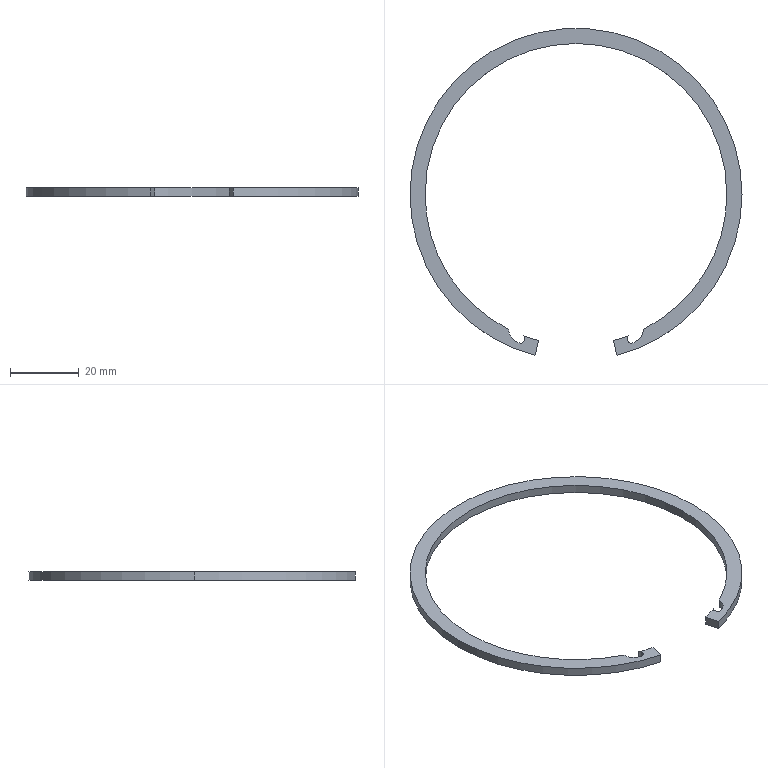Part | STEP file | Snap ring | 1 solid | 17 faces | box 96.5 x 95.005 x 2.5 mm | volume 2880 mm3 | cylinder 11 | plane 4 | spline 2 | commonest cylinder face diameters 87.7 x5 2.5 x3 96.5 x3
STEP:
#1=CARTESIAN_POINT('',(0.,0.,0.));
#2=DIRECTION('',(0.,0.,1.));
#3=DIRECTION('',(1.,0.,0.));
#4=AXIS2_PLACEMENT_3D('',#1,#2,#3);
#5=CARTESIAN_POINT('',(48.25,0.,2.5));
#6=VERTEX_POINT('',#5);
#7=CARTESIAN_POINT('',(-48.25,0.,2.5));
#8=VERTEX_POINT('',#7);
#9=CARTESIAN_POINT('',(0.,0.,2.5));
#10=DIRECTION('',(0.,0.,1.));
#11=DIRECTION('',(-1.,0.,0.));
#12=AXIS2_PLACEMENT_3D('',#9,#10,#11);
#13=CIRCLE('',#12,48.25);
#14=CARTESIAN_POINT('',(0.,0.,2.5));
#15=DIRECTION('',(0.,0.,-1.));
#16=DIRECTION('',(-1.,0.,0.));
#17=AXIS2_PLACEMENT_3D('',#14,#15,#16);
#18=CYLINDRICAL_SURFACE('',#17,48.25);
#19=CARTESIAN_POINT('',(6.283,0.));
#20=DIRECTION('',(-1.,0.));
#21=VECTOR('',#20,1.);
#22=LINE('',#19,#21);
#23=(GEOMETRIC_REPRESENTATION_CONTEXT(2)PARAMETRIC_REPRESENTATION_CONTEXT()REPRESENTATION_CONTEXT('',''));
#24=DEFINITIONAL_REPRESENTATION('',(#22),#23);
#25=PCURVE('',#18,#24);
#26=CARTESIAN_POINT('',(0.,0.,2.5));
#27=DIRECTION('',(0.,0.,1.));
#28=DIRECTION('',(1.,0.,0.));
#29=AXIS2_PLACEMENT_3D('',#26,#27,#28);
#30=PLANE('',#29);
#31=CARTESIAN_POINT('',(0.,0.));
#32=DIRECTION('',(-1.,0.));
#33=AXIS2_PLACEMENT_2D('',#31,#32);
#34=CIRCLE('',#33,48.25);
#35=(GEOMETRIC_REPRESENTATION_CONTEXT(2)PARAMETRIC_REPRESENTATION_CONTEXT()REPRESENTATION_CONTEXT('',''));
#36=DEFINITIONAL_REPRESENTATION('',(#34),#35);
#37=PCURVE('',#30,#36);
#38=SURFACE_CURVE('',#13,(#25,#37),.PCURVE_S1.);
#39=EDGE_CURVE('',#6,#8,#38,.T.);
#40=ORIENTED_EDGE('',*,*,#39,.F.);
#41=CARTESIAN_POINT('',(48.25,0.,0.));
#42=VERTEX_POINT('',#41);
#43=CARTESIAN_POINT('',(48.25,0.,2.5));
#44=DIRECTION('',(0.,0.,-1.));
#45=VECTOR('',#44,1.);
#46=LINE('',#43,#45);
#47=CARTESIAN_POINT('',(3.142,0.));
#48=DIRECTION('',(0.,1.));
#49=VECTOR('',#48,1.);
#50=LINE('',#47,#49);
#51=(GEOMETRIC_REPRESENTATION_CONTEXT(2)PARAMETRIC_REPRESENTATION_CONTEXT()REPRESENTATION_CONTEXT('',''));
#52=DEFINITIONAL_REPRESENTATION('',(#50),#51);
#53=PCURVE('',#18,#52);
#54=CARTESIAN_POINT('',(0.,0.,2.5));
#55=DIRECTION('',(0.,0.,-1.));
#56=DIRECTION('',(-1.,0.,0.));
#57=AXIS2_PLACEMENT_3D('',#54,#55,#56);
#58=CYLINDRICAL_SURFACE('',#57,48.25);
#59=CARTESIAN_POINT('',(3.142,0.));
#60=DIRECTION('',(0.,1.));
#61=VECTOR('',#60,1.);
#62=LINE('',#59,#61);
#63=(GEOMETRIC_REPRESENTATION_CONTEXT(2)PARAMETRIC_REPRESENTATION_CONTEXT()REPRESENTATION_CONTEXT('',''));
#64=DEFINITIONAL_REPRESENTATION('',(#62),#63);
#65=PCURVE('',#58,#64);
#66=SURFACE_CURVE('',#46,(#53,#65),.PCURVE_S1.);
#67=EDGE_CURVE('',#6,#42,#66,.T.);
#68=ORIENTED_EDGE('',*,*,#67,.T.);
#69=CARTESIAN_POINT('',(-48.25,0.,0.));
#70=VERTEX_POINT('',#69);
#71=CARTESIAN_POINT('',(0.,0.,0.));
#72=DIRECTION('',(0.,0.,1.));
#73=DIRECTION('',(-1.,0.,0.));
#74=AXIS2_PLACEMENT_3D('',#71,#72,#73);
#75=CIRCLE('',#74,48.25);
#76=CARTESIAN_POINT('',(6.283,2.5));
#77=DIRECTION('',(-1.,0.));
#78=VECTOR('',#77,1.);
#79=LINE('',#76,#78);
#80=(GEOMETRIC_REPRESENTATION_CONTEXT(2)PARAMETRIC_REPRESENTATION_CONTEXT()REPRESENTATION_CONTEXT('',''));
#81=DEFINITIONAL_REPRESENTATION('',(#79),#80);
#82=PCURVE('',#18,#81);
#83=CARTESIAN_POINT('',(0.,0.,0.));
#84=DIRECTION('',(0.,0.,1.));
#85=DIRECTION('',(1.,0.,0.));
#86=AXIS2_PLACEMENT_3D('',#83,#84,#85);
#87=PLANE('',#86);
#88=CARTESIAN_POINT('',(0.,0.));
#89=DIRECTION('',(-1.,0.));
#90=AXIS2_PLACEMENT_2D('',#88,#89);
#91=CIRCLE('',#90,48.25);
#92=(GEOMETRIC_REPRESENTATION_CONTEXT(2)PARAMETRIC_REPRESENTATION_CONTEXT()REPRESENTATION_CONTEXT('',''));
#93=DEFINITIONAL_REPRESENTATION('',(#91),#92);
#94=PCURVE('',#87,#93);
#95=SURFACE_CURVE('',#75,(#82,#94),.PCURVE_S1.);
#96=EDGE_CURVE('',#42,#70,#95,.T.);
#97=ORIENTED_EDGE('',*,*,#96,.T.);
#98=CARTESIAN_POINT('',(-48.25,0.,2.5));
#99=DIRECTION('',(0.,0.,-1.));
#100=VECTOR('',#99,1.);
#101=LINE('',#98,#100);
#102=CARTESIAN_POINT('',(0.,0.));
#103=DIRECTION('',(0.,1.));
#104=VECTOR('',#103,1.);
#105=LINE('',#102,#104);
#106=(GEOMETRIC_REPRESENTATION_CONTEXT(2)PARAMETRIC_REPRESENTATION_CONTEXT()REPRESENTATION_CONTEXT('',''));
#107=DEFINITIONAL_REPRESENTATION('',(#105),#106);
#108=PCURVE('',#18,#107);
#109=CARTESIAN_POINT('',(0.,0.,2.5));
#110=DIRECTION('',(0.,0.,-1.));
#111=DIRECTION('',(-1.,0.,0.));
#112=AXIS2_PLACEMENT_3D('',#109,#110,#111);
#113=CYLINDRICAL_SURFACE('',#112,48.25);
#114=CARTESIAN_POINT('',(6.283,0.));
#115=DIRECTION('',(0.,1.));
#116=VECTOR('',#115,1.);
#117=LINE('',#114,#116);
#118=(GEOMETRIC_REPRESENTATION_CONTEXT(2)PARAMETRIC_REPRESENTATION_CONTEXT()REPRESENTATION_CONTEXT('',''));
#119=DEFINITIONAL_REPRESENTATION('',(#117),#118);
#120=PCURVE('',#113,#119);
#121=SURFACE_CURVE('',#101,(#108,#120),.PCURVE_S1.);
#122=EDGE_CURVE('',#8,#70,#121,.T.);
#123=ORIENTED_EDGE('',*,*,#122,.F.);
#124=EDGE_LOOP('',(#40,#68,#97,#123));
#125=FACE_BOUND('',#124,.T.);
#126=ADVANCED_FACE('',(#125),#18,.T.);
#127=CARTESIAN_POINT('',(-11.918,-46.755,2.5));
#128=VERTEX_POINT('',#127);
#129=CARTESIAN_POINT('',(0.,0.,2.5));
#130=DIRECTION('',(0.,0.,1.));
#131=DIRECTION('',(-1.,0.,0.));
#132=AXIS2_PLACEMENT_3D('',#129,#130,#131);
#133=CIRCLE('',#132,48.25);
#134=CARTESIAN_POINT('',(6.283,0.));
#135=DIRECTION('',(-1.,0.));
#136=VECTOR('',#135,1.);
#137=LINE('',#134,#136);
#138=(GEOMETRIC_REPRESENTATION_CONTEXT(2)PARAMETRIC_REPRESENTATION_CONTEXT()REPRESENTATION_CONTEXT('',''));
#139=DEFINITIONAL_REPRESENTATION('',(#137),#138);
#140=PCURVE('',#113,#139);
#141=CARTESIAN_POINT('',(0.,0.));
#142=DIRECTION('',(-1.,0.));
#143=AXIS2_PLACEMENT_2D('',#141,#142);
#144=CIRCLE('',#143,48.25);
#145=(GEOMETRIC_REPRESENTATION_CONTEXT(2)PARAMETRIC_REPRESENTATION_CONTEXT()REPRESENTATION_CONTEXT('',''));
#146=DEFINITIONAL_REPRESENTATION('',(#144),#145);
#147=PCURVE('',#30,#146);
#148=SURFACE_CURVE('',#133,(#140,#147),.PCURVE_S1.);
#149=EDGE_CURVE('',#8,#128,#148,.T.);
#150=ORIENTED_EDGE('',*,*,#149,.F.);
#151=ORIENTED_EDGE('',*,*,#122,.T.);
#152=CARTESIAN_POINT('',(-11.918,-46.755,0.));
#153=VERTEX_POINT('',#152);
#154=CARTESIAN_POINT('',(0.,0.,0.));
#155=DIRECTION('',(0.,0.,1.));
#156=DIRECTION('',(-1.,0.,0.));
#157=AXIS2_PLACEMENT_3D('',#154,#155,#156);
#158=CIRCLE('',#157,48.25);
#159=CARTESIAN_POINT('',(6.283,2.5));
#160=DIRECTION('',(-1.,0.));
#161=VECTOR('',#160,1.);
#162=LINE('',#159,#161);
#163=(GEOMETRIC_REPRESENTATION_CONTEXT(2)PARAMETRIC_REPRESENTATION_CONTEXT()REPRESENTATION_CONTEXT('',''));
#164=DEFINITIONAL_REPRESENTATION('',(#162),#163);
#165=PCURVE('',#113,#164);
#166=CARTESIAN_POINT('',(0.,0.));
#167=DIRECTION('',(-1.,0.));
#168=AXIS2_PLACEMENT_2D('',#166,#167);
#169=CIRCLE('',#168,48.25);
#170=(GEOMETRIC_REPRESENTATION_CONTEXT(2)PARAMETRIC_REPRESENTATION_CONTEXT()REPRESENTATION_CONTEXT('',''));
#171=DEFINITIONAL_REPRESENTATION('',(#169),#170);
#172=PCURVE('',#87,#171);
#173=SURFACE_CURVE('',#158,(#165,#172),.PCURVE_S1.);
#174=EDGE_CURVE('',#70,#153,#173,.T.);
#175=ORIENTED_EDGE('',*,*,#174,.T.);
#176=CARTESIAN_POINT('',(-11.918,-46.755,2.5));
#177=DIRECTION('',(0.,0.,1.));
#178=VECTOR('',#177,1.);
#179=LINE('',#176,#178);
#180=CARTESIAN_POINT('',(4.962,0.));
#181=DIRECTION('',(0.,-1.));
#182=VECTOR('',#181,1.);
#183=LINE('',#180,#182);
#184=(GEOMETRIC_REPRESENTATION_CONTEXT(2)PARAMETRIC_REPRESENTATION_CONTEXT()REPRESENTATION_CONTEXT('',''));
#185=DEFINITIONAL_REPRESENTATION('',(#183),#184);
#186=PCURVE('',#113,#185);
#187=CARTESIAN_POINT('',(-10.831,-42.491,2.5));
#188=DIRECTION('',(-0.969,0.247,0.));
#189=DIRECTION('',(-0.247,-0.969,0.));
#190=AXIS2_PLACEMENT_3D('',#187,#188,#189);
#191=PLANE('',#190);
#192=CARTESIAN_POINT('',(4.4,0.));
#193=DIRECTION('',(0.,1.));
#194=VECTOR('',#193,1.);
#195=LINE('',#192,#194);
#196=(GEOMETRIC_REPRESENTATION_CONTEXT(2)PARAMETRIC_REPRESENTATION_CONTEXT()REPRESENTATION_CONTEXT('',''));
#197=DEFINITIONAL_REPRESENTATION('',(#195),#196);
#198=PCURVE('',#191,#197);
#199=SURFACE_CURVE('',#179,(#186,#198),.PCURVE_S1.);
#200=EDGE_CURVE('',#153,#128,#199,.T.);
#201=ORIENTED_EDGE('',*,*,#200,.T.);
#202=EDGE_LOOP('',(#150,#151,#175,#201));
#203=FACE_BOUND('',#202,.T.);
#204=ADVANCED_FACE('',(#203),#113,.T.);
#205=CARTESIAN_POINT('',(19.612,-39.22,0.));
#206=VERTEX_POINT('',#205);
#207=CARTESIAN_POINT('',(19.612,-39.22,2.5));
#208=VERTEX_POINT('',#207);
#209=CARTESIAN_POINT('',(19.612,-39.22,1.25));
#210=DIRECTION('',(0.,0.,1.));
#211=VECTOR('',#210,1.);
#212=LINE('',#209,#211);
#213=CARTESIAN_POINT('',(0.,0.,2.5));
#214=DIRECTION('',(0.,0.,-1.));
#215=DIRECTION('',(-1.,0.,0.));
#216=AXIS2_PLACEMENT_3D('',#213,#214,#215);
#217=CYLINDRICAL_SURFACE('',#216,43.85);
#218=CARTESIAN_POINT('',(4.249,1.25));
#219=DIRECTION('',(0.,-1.));
#220=VECTOR('',#219,1.);
#221=LINE('',#218,#220);
#222=(GEOMETRIC_REPRESENTATION_CONTEXT(2)PARAMETRIC_REPRESENTATION_CONTEXT()REPRESENTATION_CONTEXT('',''));
#223=DEFINITIONAL_REPRESENTATION('',(#221),#222);
#224=PCURVE('',#217,#223);
#225=CARTESIAN_POINT('',(16.56,-43.184,0.));
#226=CARTESIAN_POINT('',(16.56,-43.184,2.5));
#227=CARTESIAN_POINT('',(19.402,-42.149,0.));
#228=CARTESIAN_POINT('',(19.402,-42.149,2.5));
#229=CARTESIAN_POINT('',(19.612,-39.22,0.));
#230=CARTESIAN_POINT('',(19.612,-39.22,2.5));
#231=B_SPLINE_SURFACE_WITH_KNOTS('',2,1,((#225,#226),(#227,#228),(#229,#230)),.UNSPECIFIED.,.F.,.F.,.F.,(3,3),(2,2),(0.,1.),(0.,1.),.PIECEWISE_BEZIER_KNOTS.);
#232=CARTESIAN_POINT('',(1.,0.));
#233=CARTESIAN_POINT('',(1.,1.));
#234=B_SPLINE_CURVE_WITH_KNOTS('',1,(#232,#233),.UNSPECIFIED.,.F.,.F.,(2,2),(-1.25,1.25),.PIECEWISE_BEZIER_KNOTS.);
#235=(GEOMETRIC_REPRESENTATION_CONTEXT(2)PARAMETRIC_REPRESENTATION_CONTEXT()REPRESENTATION_CONTEXT('',''));
#236=DEFINITIONAL_REPRESENTATION('',(#234),#235);
#237=PCURVE('',#231,#236);
#238=SURFACE_CURVE('',#212,(#224,#237),.PCURVE_S1.);
#239=EDGE_CURVE('',#206,#208,#238,.T.);
#240=ORIENTED_EDGE('',*,*,#239,.F.);
#241=CARTESIAN_POINT('',(43.85,0.,0.));
#242=VERTEX_POINT('',#241);
#243=CARTESIAN_POINT('',(0.,0.,0.));
#244=DIRECTION('',(0.,0.,1.));
#245=DIRECTION('',(-1.,0.,0.));
#246=AXIS2_PLACEMENT_3D('',#243,#244,#245);
#247=CIRCLE('',#246,43.85);
#248=CARTESIAN_POINT('',(6.283,2.5));
#249=DIRECTION('',(-1.,0.));
#250=VECTOR('',#249,1.);
#251=LINE('',#248,#250);
#252=(GEOMETRIC_REPRESENTATION_CONTEXT(2)PARAMETRIC_REPRESENTATION_CONTEXT()REPRESENTATION_CONTEXT('',''));
#253=DEFINITIONAL_REPRESENTATION('',(#251),#252);
#254=PCURVE('',#217,#253);
#255=CARTESIAN_POINT('',(0.,0.));
#256=DIRECTION('',(-1.,0.));
#257=AXIS2_PLACEMENT_2D('',#255,#256);
#258=CIRCLE('',#257,43.85);
#259=(GEOMETRIC_REPRESENTATION_CONTEXT(2)PARAMETRIC_REPRESENTATION_CONTEXT()REPRESENTATION_CONTEXT('',''));
#260=DEFINITIONAL_REPRESENTATION('',(#258),#259);
#261=PCURVE('',#87,#260);
#262=SURFACE_CURVE('',#247,(#254,#261),.PCURVE_S1.);
#263=EDGE_CURVE('',#206,#242,#262,.T.);
#264=ORIENTED_EDGE('',*,*,#263,.T.);
#265=CARTESIAN_POINT('',(43.85,0.,2.5));
#266=VERTEX_POINT('',#265);
#267=CARTESIAN_POINT('',(43.85,0.,2.5));
#268=DIRECTION('',(0.,0.,-1.));
#269=VECTOR('',#268,1.);
#270=LINE('',#267,#269);
#271=CARTESIAN_POINT('',(3.142,0.));
#272=DIRECTION('',(0.,1.));
#273=VECTOR('',#272,1.);
#274=LINE('',#271,#273);
#275=(GEOMETRIC_REPRESENTATION_CONTEXT(2)PARAMETRIC_REPRESENTATION_CONTEXT()REPRESENTATION_CONTEXT('',''));
#276=DEFINITIONAL_REPRESENTATION('',(#274),#275);
#277=PCURVE('',#217,#276);
#278=CARTESIAN_POINT('',(0.,0.,2.5));
#279=DIRECTION('',(0.,0.,-1.));
#280=DIRECTION('',(-1.,0.,0.));
#281=AXIS2_PLACEMENT_3D('',#278,#279,#280);
#282=CYLINDRICAL_SURFACE('',#281,43.85);
#283=CARTESIAN_POINT('',(3.142,0.));
#284=DIRECTION('',(0.,1.));
#285=VECTOR('',#284,1.);
#286=LINE('',#283,#285);
#287=(GEOMETRIC_REPRESENTATION_CONTEXT(2)PARAMETRIC_REPRESENTATION_CONTEXT()REPRESENTATION_CONTEXT('',''));
#288=DEFINITIONAL_REPRESENTATION('',(#286),#287);
#289=PCURVE('',#282,#288);
#290=SURFACE_CURVE('',#270,(#277,#289),.PCURVE_S1.);
#291=EDGE_CURVE('',#266,#242,#290,.T.);
#292=ORIENTED_EDGE('',*,*,#291,.F.);
#293=CARTESIAN_POINT('',(0.,0.,2.5));
#294=DIRECTION('',(0.,0.,-1.));
#295=DIRECTION('',(-1.,0.,0.));
#296=AXIS2_PLACEMENT_3D('',#293,#294,#295);
#297=CIRCLE('',#296,43.85);
#298=CARTESIAN_POINT('',(0.,0.));
#299=DIRECTION('',(1.,0.));
#300=VECTOR('',#299,1.);
#301=LINE('',#298,#300);
#302=(GEOMETRIC_REPRESENTATION_CONTEXT(2)PARAMETRIC_REPRESENTATION_CONTEXT()REPRESENTATION_CONTEXT('',''));
#303=DEFINITIONAL_REPRESENTATION('',(#301),#302);
#304=PCURVE('',#217,#303);
#305=CARTESIAN_POINT('',(-43.85,0.));
#306=CARTESIAN_POINT('',(-43.85,75.95));
#307=CARTESIAN_POINT('',(21.925,37.975));
#308=CARTESIAN_POINT('',(87.7,0.));
#309=CARTESIAN_POINT('',(21.925,-37.975));
#310=CARTESIAN_POINT('',(-43.85,-75.95));
#311=CARTESIAN_POINT('',(-43.85,0.));
#312=(BOUNDED_CURVE()B_SPLINE_CURVE(2,(#305,#306,#307,#308,#309,#310,#311),.UNSPECIFIED.,.T.,.F.)B_SPLINE_CURVE_WITH_KNOTS((1,2,2,2,2,1),(-2.094,0.,2.094,4.189,6.283,8.378),.UNSPECIFIED.)CURVE()GEOMETRIC_REPRESENTATION_ITEM()RATIONAL_B_SPLINE_CURVE((1.,0.5,1.,0.5,1.,0.5,1.))REPRESENTATION_ITEM(''));
#313=(GEOMETRIC_REPRESENTATION_CONTEXT(2)PARAMETRIC_REPRESENTATION_CONTEXT()REPRESENTATION_CONTEXT('',''));
#314=DEFINITIONAL_REPRESENTATION('',(#312),#313);
#315=PCURVE('',#30,#314);
#316=SURFACE_CURVE('',#297,(#304,#315),.PCURVE_S1.);
#317=EDGE_CURVE('',#266,#208,#316,.T.);
#318=ORIENTED_EDGE('',*,*,#317,.T.);
#319=EDGE_LOOP('',(#240,#264,#292,#318));
#320=FACE_BOUND('',#319,.F.);
#321=ADVANCED_FACE('',(#320),#217,.F.);
#322=CARTESIAN_POINT('',(-43.85,0.,0.));
#323=VERTEX_POINT('',#322);
#324=CARTESIAN_POINT('',(0.,0.,0.));
#325=DIRECTION('',(0.,0.,1.));
#326=DIRECTION('',(-1.,0.,0.));
#327=AXIS2_PLACEMENT_3D('',#324,#325,#326);
#328=CIRCLE('',#327,43.85);
#329=CARTESIAN_POINT('',(6.283,2.5));
#330=DIRECTION('',(-1.,0.));
#331=VECTOR('',#330,1.);
#332=LINE('',#329,#331);
#333=(GEOMETRIC_REPRESENTATION_CONTEXT(2)PARAMETRIC_REPRESENTATION_CONTEXT()REPRESENTATION_CONTEXT('',''));
#334=DEFINITIONAL_REPRESENTATION('',(#332),#333);
#335=PCURVE('',#282,#334);
#336=CARTESIAN_POINT('',(0.,0.));
#337=DIRECTION('',(-1.,0.));
#338=AXIS2_PLACEMENT_2D('',#336,#337);
#339=CIRCLE('',#338,43.85);
#340=(GEOMETRIC_REPRESENTATION_CONTEXT(2)PARAMETRIC_REPRESENTATION_CONTEXT()REPRESENTATION_CONTEXT('',''));
#341=DEFINITIONAL_REPRESENTATION('',(#339),#340);
#342=PCURVE('',#87,#341);
#343=SURFACE_CURVE('',#328,(#335,#342),.PCURVE_S1.);
#344=EDGE_CURVE('',#242,#323,#343,.T.);
#345=ORIENTED_EDGE('',*,*,#344,.T.);
#346=CARTESIAN_POINT('',(-43.85,0.,2.5));
#347=VERTEX_POINT('',#346);
#348=CARTESIAN_POINT('',(-43.85,0.,2.5));
#349=DIRECTION('',(0.,0.,-1.));
#350=VECTOR('',#349,1.);
#351=LINE('',#348,#350);
#352=CARTESIAN_POINT('',(0.,0.));
#353=DIRECTION('',(0.,1.));
#354=VECTOR('',#353,1.);
#355=LINE('',#352,#354);
#356=(GEOMETRIC_REPRESENTATION_CONTEXT(2)PARAMETRIC_REPRESENTATION_CONTEXT()REPRESENTATION_CONTEXT('',''));
#357=DEFINITIONAL_REPRESENTATION('',(#355),#356);
#358=PCURVE('',#282,#357);
#359=CARTESIAN_POINT('',(0.,0.,2.5));
#360=DIRECTION('',(0.,0.,-1.));
#361=DIRECTION('',(-1.,0.,0.));
#362=AXIS2_PLACEMENT_3D('',#359,#360,#361);
#363=CYLINDRICAL_SURFACE('',#362,43.85);
#364=CARTESIAN_POINT('',(6.283,0.));
#365=DIRECTION('',(0.,1.));
#366=VECTOR('',#365,1.);
#367=LINE('',#364,#366);
#368=(GEOMETRIC_REPRESENTATION_CONTEXT(2)PARAMETRIC_REPRESENTATION_CONTEXT()REPRESENTATION_CONTEXT('',''));
#369=DEFINITIONAL_REPRESENTATION('',(#367),#368);
#370=PCURVE('',#363,#369);
#371=SURFACE_CURVE('',#351,(#358,#370),.PCURVE_S1.);
#372=EDGE_CURVE('',#347,#323,#371,.T.);
#373=ORIENTED_EDGE('',*,*,#372,.F.);
#374=CARTESIAN_POINT('',(0.,0.,2.5));
#375=DIRECTION('',(0.,0.,-1.));
#376=DIRECTION('',(-1.,0.,0.));
#377=AXIS2_PLACEMENT_3D('',#374,#375,#376);
#378=CIRCLE('',#377,43.85);
#379=CARTESIAN_POINT('',(0.,0.));
#380=DIRECTION('',(1.,0.));
#381=VECTOR('',#380,1.);
#382=LINE('',#379,#381);
#383=(GEOMETRIC_REPRESENTATION_CONTEXT(2)PARAMETRIC_REPRESENTATION_CONTEXT()REPRESENTATION_CONTEXT('',''));
#384=DEFINITIONAL_REPRESENTATION('',(#382),#383);
#385=PCURVE('',#282,#384);
#386=CARTESIAN_POINT('',(-43.85,0.));
#387=CARTESIAN_POINT('',(-43.85,75.95));
#388=CARTESIAN_POINT('',(21.925,37.975));
#389=CARTESIAN_POINT('',(87.7,0.));
#390=CARTESIAN_POINT('',(21.925,-37.975));
#391=CARTESIAN_POINT('',(-43.85,-75.95));
#392=CARTESIAN_POINT('',(-43.85,0.));
#393=(BOUNDED_CURVE()B_SPLINE_CURVE(2,(#386,#387,#388,#389,#390,#391,#392),.UNSPECIFIED.,.T.,.F.)B_SPLINE_CURVE_WITH_KNOTS((1,2,2,2,2,1),(-2.094,0.,2.094,4.189,6.283,8.378),.UNSPECIFIED.)CURVE()GEOMETRIC_REPRESENTATION_ITEM()RATIONAL_B_SPLINE_CURVE((1.,0.5,1.,0.5,1.,0.5,1.))REPRESENTATION_ITEM(''));
#394=(GEOMETRIC_REPRESENTATION_CONTEXT(2)PARAMETRIC_REPRESENTATION_CONTEXT()REPRESENTATION_CONTEXT('',''));
#395=DEFINITIONAL_REPRESENTATION('',(#393),#394);
#396=PCURVE('',#30,#395);
#397=SURFACE_CURVE('',#378,(#385,#396),.PCURVE_S1.);
#398=EDGE_CURVE('',#347,#266,#397,.T.);
#399=ORIENTED_EDGE('',*,*,#398,.T.);
#400=ORIENTED_EDGE('',*,*,#291,.T.);
#401=EDGE_LOOP('',(#345,#373,#399,#400));
#402=FACE_BOUND('',#401,.F.);
#403=ADVANCED_FACE('',(#402),#282,.F.);
#404=CARTESIAN_POINT('',(-15.262,-41.108,2.5));
#405=VERTEX_POINT('',#404);
#406=CARTESIAN_POINT('',(-15.262,-41.108,0.));
#407=VERTEX_POINT('',#406);
#408=CARTESIAN_POINT('',(-15.262,-41.108,2.5));
#409=DIRECTION('',(0.,0.,-1.));
#410=VECTOR('',#409,1.);
#411=LINE('',#408,#410);
#412=CARTESIAN_POINT('',(-16.126,-42.011,0.));
#413=DIRECTION('',(0.,0.,1.));
#414=DIRECTION('',(1.,0.,0.));
#415=AXIS2_PLACEMENT_3D('',#412,#413,#414);
#416=CYLINDRICAL_SURFACE('',#415,1.25);
#417=CARTESIAN_POINT('',(0.807,2.5));
#418=DIRECTION('',(0.,-1.));
#419=VECTOR('',#418,1.);
#420=LINE('',#417,#419);
#421=(GEOMETRIC_REPRESENTATION_CONTEXT(2)PARAMETRIC_REPRESENTATION_CONTEXT()REPRESENTATION_CONTEXT('',''));
#422=DEFINITIONAL_REPRESENTATION('',(#420),#421);
#423=PCURVE('',#416,#422);
#424=CARTESIAN_POINT('',(0.,0.,2.5));
#425=DIRECTION('',(0.,0.,-1.));
#426=DIRECTION('',(-1.,0.,0.));
#427=AXIS2_PLACEMENT_3D('',#424,#425,#426);
#428=CYLINDRICAL_SURFACE('',#427,43.85);
#429=CARTESIAN_POINT('',(5.068,0.));
#430=DIRECTION('',(0.,1.));
#431=VECTOR('',#430,1.);
#432=LINE('',#429,#431);
#433=(GEOMETRIC_REPRESENTATION_CONTEXT(2)PARAMETRIC_REPRESENTATION_CONTEXT()REPRESENTATION_CONTEXT('',''));
#434=DEFINITIONAL_REPRESENTATION('',(#432),#433);
#435=PCURVE('',#428,#434);
#436=SURFACE_CURVE('',#411,(#423,#435),.PCURVE_S1.);
#437=EDGE_CURVE('',#405,#407,#436,.T.);
#438=ORIENTED_EDGE('',*,*,#437,.F.);
#439=CARTESIAN_POINT('',(-14.876,-42.011,2.5));
#440=VERTEX_POINT('',#439);
#441=CARTESIAN_POINT('',(-16.126,-42.011,2.5));
#442=DIRECTION('',(0.,0.,-1.));
#443=DIRECTION('',(1.,0.,0.));
#444=AXIS2_PLACEMENT_3D('',#441,#442,#443);
#445=CIRCLE('',#444,1.25);
#446=CARTESIAN_POINT('',(6.283,2.5));
#447=DIRECTION('',(-1.,0.));
#448=VECTOR('',#447,1.);
#449=LINE('',#446,#448);
#450=(GEOMETRIC_REPRESENTATION_CONTEXT(2)PARAMETRIC_REPRESENTATION_CONTEXT()REPRESENTATION_CONTEXT('',''));
#451=DEFINITIONAL_REPRESENTATION('',(#449),#450);
#452=PCURVE('',#416,#451);
#453=CARTESIAN_POINT('',(-14.876,-42.011));
#454=CARTESIAN_POINT('',(-14.876,-44.176));
#455=CARTESIAN_POINT('',(-16.751,-43.094));
#456=CARTESIAN_POINT('',(-18.626,-42.011));
#457=CARTESIAN_POINT('',(-16.751,-40.929));
#458=CARTESIAN_POINT('',(-14.876,-39.846));
#459=CARTESIAN_POINT('',(-14.876,-42.011));
#460=(BOUNDED_CURVE()B_SPLINE_CURVE(2,(#453,#454,#455,#456,#457,#458,#459),.UNSPECIFIED.,.T.,.F.)B_SPLINE_CURVE_WITH_KNOTS((1,2,2,2,2,1),(-2.094,0.,2.094,4.189,6.283,8.378),.UNSPECIFIED.)CURVE()GEOMETRIC_REPRESENTATION_ITEM()RATIONAL_B_SPLINE_CURVE((1.,0.5,1.,0.5,1.,0.5,1.))REPRESENTATION_ITEM(''));
#461=(GEOMETRIC_REPRESENTATION_CONTEXT(2)PARAMETRIC_REPRESENTATION_CONTEXT()REPRESENTATION_CONTEXT('',''));
#462=DEFINITIONAL_REPRESENTATION('',(#460),#461);
#463=PCURVE('',#30,#462);
#464=SURFACE_CURVE('',#445,(#452,#463),.PCURVE_S1.);
#465=EDGE_CURVE('',#405,#440,#464,.T.);
#466=ORIENTED_EDGE('',*,*,#465,.T.);
#467=CARTESIAN_POINT('',(-14.876,-42.011,0.));
#468=VERTEX_POINT('',#467);
#469=CARTESIAN_POINT('',(-14.876,-42.011,0.));
#470=DIRECTION('',(0.,0.,1.));
#471=VECTOR('',#470,1.);
#472=LINE('',#469,#471);
#473=CARTESIAN_POINT('',(0.,0.));
#474=DIRECTION('',(0.,1.));
#475=VECTOR('',#474,1.);
#476=LINE('',#473,#475);
#477=(GEOMETRIC_REPRESENTATION_CONTEXT(2)PARAMETRIC_REPRESENTATION_CONTEXT()REPRESENTATION_CONTEXT('',''));
#478=DEFINITIONAL_REPRESENTATION('',(#476),#477);
#479=PCURVE('',#416,#478);
#480=CARTESIAN_POINT('',(-16.126,-42.011,0.));
#481=DIRECTION('',(0.,0.,1.));
#482=DIRECTION('',(1.,0.,0.));
#483=AXIS2_PLACEMENT_3D('',#480,#481,#482);
#484=CYLINDRICAL_SURFACE('',#483,1.25);
#485=CARTESIAN_POINT('',(6.283,0.));
#486=DIRECTION('',(0.,1.));
#487=VECTOR('',#486,1.);
#488=LINE('',#485,#487);
#489=(GEOMETRIC_REPRESENTATION_CONTEXT(2)PARAMETRIC_REPRESENTATION_CONTEXT()REPRESENTATION_CONTEXT('',''));
#490=DEFINITIONAL_REPRESENTATION('',(#488),#489);
#491=PCURVE('',#484,#490);
#492=SURFACE_CURVE('',#472,(#479,#491),.PCURVE_S1.);
#493=EDGE_CURVE('',#468,#440,#492,.T.);
#494=ORIENTED_EDGE('',*,*,#493,.F.);
#495=CARTESIAN_POINT('',(-16.126,-42.011,0.));
#496=DIRECTION('',(0.,0.,1.));
#497=DIRECTION('',(1.,0.,0.));
#498=AXIS2_PLACEMENT_3D('',#495,#496,#497);
#499=CIRCLE('',#498,1.25);
#500=CARTESIAN_POINT('',(0.,0.));
#501=DIRECTION('',(1.,0.));
#502=VECTOR('',#501,1.);
#503=LINE('',#500,#502);
#504=(GEOMETRIC_REPRESENTATION_CONTEXT(2)PARAMETRIC_REPRESENTATION_CONTEXT()REPRESENTATION_CONTEXT('',''));
#505=DEFINITIONAL_REPRESENTATION('',(#503),#504);
#506=PCURVE('',#416,#505);
#507=CARTESIAN_POINT('',(-16.126,-42.011));
#508=DIRECTION('',(1.,0.));
#509=AXIS2_PLACEMENT_2D('',#507,#508);
#510=CIRCLE('',#509,1.25);
#511=(GEOMETRIC_REPRESENTATION_CONTEXT(2)PARAMETRIC_REPRESENTATION_CONTEXT()REPRESENTATION_CONTEXT('',''));
#512=DEFINITIONAL_REPRESENTATION('',(#510),#511);
#513=PCURVE('',#87,#512);
#514=SURFACE_CURVE('',#499,(#506,#513),.PCURVE_S1.);
#515=EDGE_CURVE('',#468,#407,#514,.T.);
#516=ORIENTED_EDGE('',*,*,#515,.T.);
#517=EDGE_LOOP('',(#438,#466,#494,#516));
#518=FACE_BOUND('',#517,.F.);
#519=ADVANCED_FACE('',(#518),#416,.F.);
#520=CARTESIAN_POINT('',(-10.831,-42.491,2.5));
#521=VERTEX_POINT('',#520);
#522=CARTESIAN_POINT('',(-11.918,-46.755,2.5));
#523=DIRECTION('',(0.247,0.969,0.));
#524=VECTOR('',#523,1.);
#525=LINE('',#522,#524);
#526=CARTESIAN_POINT('',(-11.918,-46.755));
#527=DIRECTION('',(0.247,0.969));
#528=VECTOR('',#527,1.);
#529=LINE('',#526,#528);
#530=(GEOMETRIC_REPRESENTATION_CONTEXT(2)PARAMETRIC_REPRESENTATION_CONTEXT()REPRESENTATION_CONTEXT('',''));
#531=DEFINITIONAL_REPRESENTATION('',(#529),#530);
#532=PCURVE('',#30,#531);
#533=CARTESIAN_POINT('',(4.4,0.));
#534=DIRECTION('',(-1.,0.));
#535=VECTOR('',#534,1.);
#536=LINE('',#533,#535);
#537=(GEOMETRIC_REPRESENTATION_CONTEXT(2)PARAMETRIC_REPRESENTATION_CONTEXT()REPRESENTATION_CONTEXT('',''));
#538=DEFINITIONAL_REPRESENTATION('',(#536),#537);
#539=PCURVE('',#191,#538);
#540=SURFACE_CURVE('',#525,(#532,#539),.PCURVE_S1.);
#541=EDGE_CURVE('',#128,#521,#540,.T.);
#542=ORIENTED_EDGE('',*,*,#541,.T.);
#543=CARTESIAN_POINT('',(0.,0.,2.5));
#544=DIRECTION('',(0.,0.,-1.));
#545=DIRECTION('',(-1.,0.,0.));
#546=AXIS2_PLACEMENT_3D('',#543,#544,#545);
#547=CIRCLE('',#546,43.85);
#548=CARTESIAN_POINT('',(-43.85,0.));
#549=CARTESIAN_POINT('',(-43.85,75.95));
#550=CARTESIAN_POINT('',(21.925,37.975));
#551=CARTESIAN_POINT('',(87.7,0.));
#552=CARTESIAN_POINT('',(21.925,-37.975));
#553=CARTESIAN_POINT('',(-43.85,-75.95));
#554=CARTESIAN_POINT('',(-43.85,0.));
#555=(BOUNDED_CURVE()B_SPLINE_CURVE(2,(#548,#549,#550,#551,#552,#553,#554),.UNSPECIFIED.,.T.,.F.)B_SPLINE_CURVE_WITH_KNOTS((1,2,2,2,2,1),(-2.094,0.,2.094,4.189,6.283,8.378),.UNSPECIFIED.)CURVE()GEOMETRIC_REPRESENTATION_ITEM()RATIONAL_B_SPLINE_CURVE((1.,0.5,1.,0.5,1.,0.5,1.))REPRESENTATION_ITEM(''));
#556=(GEOMETRIC_REPRESENTATION_CONTEXT(2)PARAMETRIC_REPRESENTATION_CONTEXT()REPRESENTATION_CONTEXT('',''));
#557=DEFINITIONAL_REPRESENTATION('',(#555),#556);
#558=PCURVE('',#30,#557);
#559=CARTESIAN_POINT('',(0.,0.));
#560=DIRECTION('',(1.,0.));
#561=VECTOR('',#560,1.);
#562=LINE('',#559,#561);
#563=(GEOMETRIC_REPRESENTATION_CONTEXT(2)PARAMETRIC_REPRESENTATION_CONTEXT()REPRESENTATION_CONTEXT('',''));
#564=DEFINITIONAL_REPRESENTATION('',(#562),#563);
#565=PCURVE('',#428,#564);
#566=SURFACE_CURVE('',#547,(#558,#565),.PCURVE_S1.);
#567=EDGE_CURVE('',#521,#405,#566,.T.);
#568=ORIENTED_EDGE('',*,*,#567,.T.);
#569=ORIENTED_EDGE('',*,*,#465,.T.);
#570=CARTESIAN_POINT('',(-16.56,-43.184,2.5));
#571=VERTEX_POINT('',#570);
#572=CARTESIAN_POINT('',(-16.126,-42.011,2.5));
#573=DIRECTION('',(0.,0.,-1.));
#574=DIRECTION('',(1.,0.,0.));
#575=AXIS2_PLACEMENT_3D('',#572,#573,#574);
#576=CIRCLE('',#575,1.25);
#577=CARTESIAN_POINT('',(-14.876,-42.011));
#578=CARTESIAN_POINT('',(-14.876,-44.176));
#579=CARTESIAN_POINT('',(-16.751,-43.094));
#580=CARTESIAN_POINT('',(-18.626,-42.011));
#581=CARTESIAN_POINT('',(-16.751,-40.929));
#582=CARTESIAN_POINT('',(-14.876,-39.846));
#583=CARTESIAN_POINT('',(-14.876,-42.011));
#584=(BOUNDED_CURVE()B_SPLINE_CURVE(2,(#577,#578,#579,#580,#581,#582,#583),.UNSPECIFIED.,.T.,.F.)B_SPLINE_CURVE_WITH_KNOTS((1,2,2,2,2,1),(-2.094,0.,2.094,4.189,6.283,8.378),.UNSPECIFIED.)CURVE()GEOMETRIC_REPRESENTATION_ITEM()RATIONAL_B_SPLINE_CURVE((1.,0.5,1.,0.5,1.,0.5,1.))REPRESENTATION_ITEM(''));
#585=(GEOMETRIC_REPRESENTATION_CONTEXT(2)PARAMETRIC_REPRESENTATION_CONTEXT()REPRESENTATION_CONTEXT('',''));
#586=DEFINITIONAL_REPRESENTATION('',(#584),#585);
#587=PCURVE('',#30,#586);
#588=CARTESIAN_POINT('',(6.283,2.5));
#589=DIRECTION('',(-1.,0.));
#590=VECTOR('',#589,1.);
#591=LINE('',#588,#590);
#592=(GEOMETRIC_REPRESENTATION_CONTEXT(2)PARAMETRIC_REPRESENTATION_CONTEXT()REPRESENTATION_CONTEXT('',''));
#593=DEFINITIONAL_REPRESENTATION('',(#591),#592);
#594=PCURVE('',#484,#593);
#595=SURFACE_CURVE('',#576,(#587,#594),.PCURVE_S1.);
#596=EDGE_CURVE('',#440,#571,#595,.T.);
#597=ORIENTED_EDGE('',*,*,#596,.T.);
#598=CARTESIAN_POINT('',(-19.612,-39.22,2.5));
#599=VERTEX_POINT('',#598);
#600=CARTESIAN_POINT('',(-16.56,-43.184,2.5));
#601=CARTESIAN_POINT('',(-18.454,-42.494,2.5));
#602=CARTESIAN_POINT('',(-19.472,-41.173,2.5));
#603=CARTESIAN_POINT('',(-19.612,-39.22,2.5));
#604=B_SPLINE_CURVE_WITH_KNOTS('',3,(#600,#601,#602,#603),.UNSPECIFIED.,.F.,.F.,(4,4),(0.,1.),.PIECEWISE_BEZIER_KNOTS.);
#605=CARTESIAN_POINT('',(-16.56,-43.184));
#606=CARTESIAN_POINT('',(-18.454,-42.494));
#607=CARTESIAN_POINT('',(-19.472,-41.173));
#608=CARTESIAN_POINT('',(-19.612,-39.22));
#609=B_SPLINE_CURVE_WITH_KNOTS('',3,(#605,#606,#607,#608),.UNSPECIFIED.,.F.,.F.,(4,4),(0.,1.),.PIECEWISE_BEZIER_KNOTS.);
#610=(GEOMETRIC_REPRESENTATION_CONTEXT(2)PARAMETRIC_REPRESENTATION_CONTEXT()REPRESENTATION_CONTEXT('',''));
#611=DEFINITIONAL_REPRESENTATION('',(#609),#610);
#612=PCURVE('',#30,#611);
#613=CARTESIAN_POINT('',(-16.56,-43.184,0.));
#614=CARTESIAN_POINT('',(-16.56,-43.184,2.5));
#615=CARTESIAN_POINT('',(-19.402,-42.149,0.));
#616=CARTESIAN_POINT('',(-19.402,-42.149,2.5));
#617=CARTESIAN_POINT('',(-19.612,-39.22,0.));
#618=CARTESIAN_POINT('',(-19.612,-39.22,2.5));
#619=B_SPLINE_SURFACE_WITH_KNOTS('',2,1,((#613,#614),(#615,#616),(#617,#618)),.UNSPECIFIED.,.F.,.F.,.F.,(3,3),(2,2),(0.,1.),(0.,1.),.PIECEWISE_BEZIER_KNOTS.);
#620=CARTESIAN_POINT('',(0.,1.));
#621=DIRECTION('',(1.,0.));
#622=VECTOR('',#621,1.);
#623=LINE('',#620,#622);
#624=(GEOMETRIC_REPRESENTATION_CONTEXT(2)PARAMETRIC_REPRESENTATION_CONTEXT()REPRESENTATION_CONTEXT('',''));
#625=DEFINITIONAL_REPRESENTATION('',(#623),#624);
#626=PCURVE('',#619,#625);
#627=SURFACE_CURVE('',#604,(#612,#626),.PCURVE_S1.);
#628=EDGE_CURVE('',#571,#599,#627,.T.);
#629=ORIENTED_EDGE('',*,*,#628,.T.);
#630=CARTESIAN_POINT('',(0.,0.,2.5));
#631=DIRECTION('',(0.,0.,-1.));
#632=DIRECTION('',(-1.,0.,0.));
#633=AXIS2_PLACEMENT_3D('',#630,#631,#632);
#634=CIRCLE('',#633,43.85);
#635=CARTESIAN_POINT('',(-43.85,0.));
#636=CARTESIAN_POINT('',(-43.85,75.95));
#637=CARTESIAN_POINT('',(21.925,37.975));
#638=CARTESIAN_POINT('',(87.7,0.));
#639=CARTESIAN_POINT('',(21.925,-37.975));
#640=CARTESIAN_POINT('',(-43.85,-75.95));
#641=CARTESIAN_POINT('',(-43.85,0.));
#642=(BOUNDED_CURVE()B_SPLINE_CURVE(2,(#635,#636,#637,#638,#639,#640,#641),.UNSPECIFIED.,.T.,.F.)B_SPLINE_CURVE_WITH_KNOTS((1,2,2,2,2,1),(-2.094,0.,2.094,4.189,6.283,8.378),.UNSPECIFIED.)CURVE()GEOMETRIC_REPRESENTATION_ITEM()RATIONAL_B_SPLINE_CURVE((1.,0.5,1.,0.5,1.,0.5,1.))REPRESENTATION_ITEM(''));
#643=(GEOMETRIC_REPRESENTATION_CONTEXT(2)PARAMETRIC_REPRESENTATION_CONTEXT()REPRESENTATION_CONTEXT('',''));
#644=DEFINITIONAL_REPRESENTATION('',(#642),#643);
#645=PCURVE('',#30,#644);
#646=CARTESIAN_POINT('',(0.,0.));
#647=DIRECTION('',(1.,0.));
#648=VECTOR('',#647,1.);
#649=LINE('',#646,#648);
#650=(GEOMETRIC_REPRESENTATION_CONTEXT(2)PARAMETRIC_REPRESENTATION_CONTEXT()REPRESENTATION_CONTEXT('',''));
#651=DEFINITIONAL_REPRESENTATION('',(#649),#650);
#652=PCURVE('',#363,#651);
#653=SURFACE_CURVE('',#634,(#645,#652),.PCURVE_S1.);
#654=EDGE_CURVE('',#599,#347,#653,.T.);
#655=ORIENTED_EDGE('',*,*,#654,.T.);
#656=ORIENTED_EDGE('',*,*,#398,.T.);
#657=ORIENTED_EDGE('',*,*,#317,.T.);
#658=CARTESIAN_POINT('',(16.56,-43.184,2.5));
#659=VERTEX_POINT('',#658);
#660=CARTESIAN_POINT('',(19.612,-39.22,2.5));
#661=CARTESIAN_POINT('',(19.472,-41.173,2.5));
#662=CARTESIAN_POINT('',(18.454,-42.494,2.5));
#663=CARTESIAN_POINT('',(16.56,-43.184,2.5));
#664=B_SPLINE_CURVE_WITH_KNOTS('',3,(#660,#661,#662,#663),.UNSPECIFIED.,.F.,.F.,(4,4),(0.,1.),.PIECEWISE_BEZIER_KNOTS.);
#665=CARTESIAN_POINT('',(19.612,-39.22));
#666=CARTESIAN_POINT('',(19.472,-41.173));
#667=CARTESIAN_POINT('',(18.454,-42.494));
#668=CARTESIAN_POINT('',(16.56,-43.184));
#669=B_SPLINE_CURVE_WITH_KNOTS('',3,(#665,#666,#667,#668),.UNSPECIFIED.,.F.,.F.,(4,4),(0.,1.),.PIECEWISE_BEZIER_KNOTS.);
#670=(GEOMETRIC_REPRESENTATION_CONTEXT(2)PARAMETRIC_REPRESENTATION_CONTEXT()REPRESENTATION_CONTEXT('',''));
#671=DEFINITIONAL_REPRESENTATION('',(#669),#670);
#672=PCURVE('',#30,#671);
#673=CARTESIAN_POINT('',(1.,1.));
#674=DIRECTION('',(-1.,0.));
#675=VECTOR('',#674,1.);
#676=LINE('',#673,#675);
#677=(GEOMETRIC_REPRESENTATION_CONTEXT(2)PARAMETRIC_REPRESENTATION_CONTEXT()REPRESENTATION_CONTEXT('',''));
#678=DEFINITIONAL_REPRESENTATION('',(#676),#677);
#679=PCURVE('',#231,#678);
#680=SURFACE_CURVE('',#664,(#672,#679),.PCURVE_S1.);
#681=EDGE_CURVE('',#208,#659,#680,.T.);
#682=ORIENTED_EDGE('',*,*,#681,.T.);
#683=CARTESIAN_POINT('',(15.262,-41.108,2.5));
#684=VERTEX_POINT('',#683);
#685=CARTESIAN_POINT('',(16.126,-42.011,2.5));
#686=DIRECTION('',(0.,0.,-1.));
#687=DIRECTION('',(1.,0.,0.));
#688=AXIS2_PLACEMENT_3D('',#685,#686,#687);
#689=CIRCLE('',#688,1.25);
#690=CARTESIAN_POINT('',(17.376,-42.011));
#691=CARTESIAN_POINT('',(17.376,-44.176));
#692=CARTESIAN_POINT('',(15.501,-43.094));
#693=CARTESIAN_POINT('',(13.626,-42.011));
#694=CARTESIAN_POINT('',(15.501,-40.929));
#695=CARTESIAN_POINT('',(17.376,-39.846));
#696=CARTESIAN_POINT('',(17.376,-42.011));
#697=(BOUNDED_CURVE()B_SPLINE_CURVE(2,(#690,#691,#692,#693,#694,#695,#696),.UNSPECIFIED.,.T.,.F.)B_SPLINE_CURVE_WITH_KNOTS((1,2,2,2,2,1),(-2.094,0.,2.094,4.189,6.283,8.378),.UNSPECIFIED.)CURVE()GEOMETRIC_REPRESENTATION_ITEM()RATIONAL_B_SPLINE_CURVE((1.,0.5,1.,0.5,1.,0.5,1.))REPRESENTATION_ITEM(''));
#698=(GEOMETRIC_REPRESENTATION_CONTEXT(2)PARAMETRIC_REPRESENTATION_CONTEXT()REPRESENTATION_CONTEXT('',''));
#699=DEFINITIONAL_REPRESENTATION('',(#697),#698);
#700=PCURVE('',#30,#699);
#701=CARTESIAN_POINT('',(16.126,-42.011,0.));
#702=DIRECTION('',(0.,0.,1.));
#703=DIRECTION('',(1.,0.,0.));
#704=AXIS2_PLACEMENT_3D('',#701,#702,#703);
#705=CYLINDRICAL_SURFACE('',#704,1.25);
#706=CARTESIAN_POINT('',(6.283,2.5));
#707=DIRECTION('',(-1.,0.));
#708=VECTOR('',#707,1.);
#709=LINE('',#706,#708);
#710=(GEOMETRIC_REPRESENTATION_CONTEXT(2)PARAMETRIC_REPRESENTATION_CONTEXT()REPRESENTATION_CONTEXT('',''));
#711=DEFINITIONAL_REPRESENTATION('',(#709),#710);
#712=PCURVE('',#705,#711);
#713=SURFACE_CURVE('',#689,(#700,#712),.PCURVE_S1.);
#714=EDGE_CURVE('',#659,#684,#713,.T.);
#715=ORIENTED_EDGE('',*,*,#714,.T.);
#716=CARTESIAN_POINT('',(10.831,-42.491,2.5));
#717=VERTEX_POINT('',#716);
#718=CARTESIAN_POINT('',(0.,0.,2.5));
#719=DIRECTION('',(0.,0.,-1.));
#720=DIRECTION('',(-1.,0.,0.));
#721=AXIS2_PLACEMENT_3D('',#718,#719,#720);
#722=CIRCLE('',#721,43.85);
#723=CARTESIAN_POINT('',(-43.85,0.));
#724=CARTESIAN_POINT('',(-43.85,75.95));
#725=CARTESIAN_POINT('',(21.925,37.975));
#726=CARTESIAN_POINT('',(87.7,0.));
#727=CARTESIAN_POINT('',(21.925,-37.975));
#728=CARTESIAN_POINT('',(-43.85,-75.95));
#729=CARTESIAN_POINT('',(-43.85,0.));
#730=(BOUNDED_CURVE()B_SPLINE_CURVE(2,(#723,#724,#725,#726,#727,#728,#729),.UNSPECIFIED.,.T.,.F.)B_SPLINE_CURVE_WITH_KNOTS((1,2,2,2,2,1),(-2.094,0.,2.094,4.189,6.283,8.378),.UNSPECIFIED.)CURVE()GEOMETRIC_REPRESENTATION_ITEM()RATIONAL_B_SPLINE_CURVE((1.,0.5,1.,0.5,1.,0.5,1.))REPRESENTATION_ITEM(''));
#731=(GEOMETRIC_REPRESENTATION_CONTEXT(2)PARAMETRIC_REPRESENTATION_CONTEXT()REPRESENTATION_CONTEXT('',''));
#732=DEFINITIONAL_REPRESENTATION('',(#730),#731);
#733=PCURVE('',#30,#732);
#734=CARTESIAN_POINT('',(0.,0.,2.5));
#735=DIRECTION('',(0.,0.,-1.));
#736=DIRECTION('',(-1.,0.,0.));
#737=AXIS2_PLACEMENT_3D('',#734,#735,#736);
#738=CYLINDRICAL_SURFACE('',#737,43.85);
#739=CARTESIAN_POINT('',(0.,0.));
#740=DIRECTION('',(1.,0.));
#741=VECTOR('',#740,1.);
#742=LINE('',#739,#741);
#743=(GEOMETRIC_REPRESENTATION_CONTEXT(2)PARAMETRIC_REPRESENTATION_CONTEXT()REPRESENTATION_CONTEXT('',''));
#744=DEFINITIONAL_REPRESENTATION('',(#742),#743);
#745=PCURVE('',#738,#744);
#746=SURFACE_CURVE('',#722,(#733,#745),.PCURVE_S1.);
#747=EDGE_CURVE('',#684,#717,#746,.T.);
#748=ORIENTED_EDGE('',*,*,#747,.T.);
#749=CARTESIAN_POINT('',(11.918,-46.755,2.5));
#750=VERTEX_POINT('',#749);
#751=CARTESIAN_POINT('',(10.831,-42.491,2.5));
#752=DIRECTION('',(0.247,-0.969,0.));
#753=VECTOR('',#752,1.);
#754=LINE('',#751,#753);
#755=CARTESIAN_POINT('',(10.831,-42.491));
#756=DIRECTION('',(0.247,-0.969));
#757=VECTOR('',#756,1.);
#758=LINE('',#755,#757);
#759=(GEOMETRIC_REPRESENTATION_CONTEXT(2)PARAMETRIC_REPRESENTATION_CONTEXT()REPRESENTATION_CONTEXT('',''));
#760=DEFINITIONAL_REPRESENTATION('',(#758),#759);
#761=PCURVE('',#30,#760);
#762=CARTESIAN_POINT('',(10.831,-42.491,2.5));
#763=DIRECTION('',(0.969,0.247,0.));
#764=DIRECTION('',(-0.247,0.969,0.));
#765=AXIS2_PLACEMENT_3D('',#762,#763,#764);
#766=PLANE('',#765);
#767=CARTESIAN_POINT('',(0.,0.));
#768=DIRECTION('',(-1.,0.));
#769=VECTOR('',#768,1.);
#770=LINE('',#767,#769);
#771=(GEOMETRIC_REPRESENTATION_CONTEXT(2)PARAMETRIC_REPRESENTATION_CONTEXT()REPRESENTATION_CONTEXT('',''));
#772=DEFINITIONAL_REPRESENTATION('',(#770),#771);
#773=PCURVE('',#766,#772);
#774=SURFACE_CURVE('',#754,(#761,#773),.PCURVE_S1.);
#775=EDGE_CURVE('',#717,#750,#774,.T.);
#776=ORIENTED_EDGE('',*,*,#775,.T.);
#777=CARTESIAN_POINT('',(0.,0.,2.5));
#778=DIRECTION('',(0.,0.,1.));
#779=DIRECTION('',(-1.,0.,0.));
#780=AXIS2_PLACEMENT_3D('',#777,#778,#779);
#781=CIRCLE('',#780,48.25);
#782=CARTESIAN_POINT('',(0.,0.));
#783=DIRECTION('',(-1.,0.));
#784=AXIS2_PLACEMENT_2D('',#782,#783);
#785=CIRCLE('',#784,48.25);
#786=(GEOMETRIC_REPRESENTATION_CONTEXT(2)PARAMETRIC_REPRESENTATION_CONTEXT()REPRESENTATION_CONTEXT('',''));
#787=DEFINITIONAL_REPRESENTATION('',(#785),#786);
#788=PCURVE('',#30,#787);
#789=CARTESIAN_POINT('',(6.283,0.));
#790=DIRECTION('',(-1.,0.));
#791=VECTOR('',#790,1.);
#792=LINE('',#789,#791);
#793=(GEOMETRIC_REPRESENTATION_CONTEXT(2)PARAMETRIC_REPRESENTATION_CONTEXT()REPRESENTATION_CONTEXT('',''));
#794=DEFINITIONAL_REPRESENTATION('',(#792),#793);
#795=PCURVE('',#58,#794);
#796=SURFACE_CURVE('',#781,(#788,#795),.PCURVE_S1.);
#797=EDGE_CURVE('',#750,#6,#796,.T.);
#798=ORIENTED_EDGE('',*,*,#797,.T.);
#799=ORIENTED_EDGE('',*,*,#39,.T.);
#800=ORIENTED_EDGE('',*,*,#149,.T.);
#801=EDGE_LOOP('',(#542,#568,#569,#597,#629,#655,#656,#657,#682,#715,#748,#776,#798,#799,#800));
#802=FACE_BOUND('',#801,.T.);
#803=ADVANCED_FACE('',(#802),#30,.T.);
#804=ORIENTED_EDGE('',*,*,#437,.T.);
#805=CARTESIAN_POINT('',(-10.831,-42.491,0.));
#806=VERTEX_POINT('',#805);
#807=CARTESIAN_POINT('',(0.,0.,0.));
#808=DIRECTION('',(0.,0.,1.));
#809=DIRECTION('',(-1.,0.,0.));
#810=AXIS2_PLACEMENT_3D('',#807,#808,#809);
#811=CIRCLE('',#810,43.85);
#812=CARTESIAN_POINT('',(6.283,2.5));
#813=DIRECTION('',(-1.,0.));
#814=VECTOR('',#813,1.);
#815=LINE('',#812,#814);
#816=(GEOMETRIC_REPRESENTATION_CONTEXT(2)PARAMETRIC_REPRESENTATION_CONTEXT()REPRESENTATION_CONTEXT('',''));
#817=DEFINITIONAL_REPRESENTATION('',(#815),#816);
#818=PCURVE('',#428,#817);
#819=CARTESIAN_POINT('',(0.,0.));
#820=DIRECTION('',(-1.,0.));
#821=AXIS2_PLACEMENT_2D('',#819,#820);
#822=CIRCLE('',#821,43.85);
#823=(GEOMETRIC_REPRESENTATION_CONTEXT(2)PARAMETRIC_REPRESENTATION_CONTEXT()REPRESENTATION_CONTEXT('',''));
#824=DEFINITIONAL_REPRESENTATION('',(#822),#823);
#825=PCURVE('',#87,#824);
#826=SURFACE_CURVE('',#811,(#818,#825),.PCURVE_S1.);
#827=EDGE_CURVE('',#407,#806,#826,.T.);
#828=ORIENTED_EDGE('',*,*,#827,.T.);
#829=CARTESIAN_POINT('',(-10.831,-42.491,2.5));
#830=DIRECTION('',(0.,0.,1.));
#831=VECTOR('',#830,1.);
#832=LINE('',#829,#831);
#833=CARTESIAN_POINT('',(4.962,0.));
#834=DIRECTION('',(0.,-1.));
#835=VECTOR('',#834,1.);
#836=LINE('',#833,#835);
#837=(GEOMETRIC_REPRESENTATION_CONTEXT(2)PARAMETRIC_REPRESENTATION_CONTEXT()REPRESENTATION_CONTEXT('',''));
#838=DEFINITIONAL_REPRESENTATION('',(#836),#837);
#839=PCURVE('',#428,#838);
#840=CARTESIAN_POINT('',(0.,0.));
#841=DIRECTION('',(0.,1.));
#842=VECTOR('',#841,1.);
#843=LINE('',#840,#842);
#844=(GEOMETRIC_REPRESENTATION_CONTEXT(2)PARAMETRIC_REPRESENTATION_CONTEXT()REPRESENTATION_CONTEXT('',''));
#845=DEFINITIONAL_REPRESENTATION('',(#843),#844);
#846=PCURVE('',#191,#845);
#847=SURFACE_CURVE('',#832,(#839,#846),.PCURVE_S1.);
#848=EDGE_CURVE('',#806,#521,#847,.T.);
#849=ORIENTED_EDGE('',*,*,#848,.T.);
#850=ORIENTED_EDGE('',*,*,#567,.T.);
#851=EDGE_LOOP('',(#804,#828,#849,#850));
#852=FACE_BOUND('',#851,.F.);
#853=ADVANCED_FACE('',(#852),#428,.F.);
#854=ORIENTED_EDGE('',*,*,#848,.T.);
#855=ORIENTED_EDGE('',*,*,#541,.F.);
#856=ORIENTED_EDGE('',*,*,#200,.F.);
#857=CARTESIAN_POINT('',(-10.831,-42.491,0.));
#858=DIRECTION('',(-0.247,-0.969,0.));
#859=VECTOR('',#858,1.);
#860=LINE('',#857,#859);
#861=CARTESIAN_POINT('',(0.,-2.5));
#862=DIRECTION('',(1.,0.));
#863=VECTOR('',#862,1.);
#864=LINE('',#861,#863);
#865=(GEOMETRIC_REPRESENTATION_CONTEXT(2)PARAMETRIC_REPRESENTATION_CONTEXT()REPRESENTATION_CONTEXT('',''));
#866=DEFINITIONAL_REPRESENTATION('',(#864),#865);
#867=PCURVE('',#191,#866);
#868=CARTESIAN_POINT('',(-10.831,-42.491));
#869=DIRECTION('',(-0.247,-0.969));
#870=VECTOR('',#869,1.);
#871=LINE('',#868,#870);
#872=(GEOMETRIC_REPRESENTATION_CONTEXT(2)PARAMETRIC_REPRESENTATION_CONTEXT()REPRESENTATION_CONTEXT('',''));
#873=DEFINITIONAL_REPRESENTATION('',(#871),#872);
#874=PCURVE('',#87,#873);
#875=SURFACE_CURVE('',#860,(#867,#874),.PCURVE_S1.);
#876=EDGE_CURVE('',#806,#153,#875,.T.);
#877=ORIENTED_EDGE('',*,*,#876,.F.);
#878=EDGE_LOOP('',(#854,#855,#856,#877));
#879=FACE_BOUND('',#878,.T.);
#880=ADVANCED_FACE('',(#879),#191,.F.);
#881=ORIENTED_EDGE('',*,*,#67,.F.);
#882=ORIENTED_EDGE('',*,*,#797,.F.);
#883=CARTESIAN_POINT('',(11.918,-46.755,0.));
#884=VERTEX_POINT('',#883);
#885=CARTESIAN_POINT('',(11.918,-46.755,2.5));
#886=DIRECTION('',(0.,0.,-1.));
#887=VECTOR('',#886,1.);
#888=LINE('',#885,#887);
#889=CARTESIAN_POINT('',(4.463,0.));
#890=DIRECTION('',(0.,1.));
#891=VECTOR('',#890,1.);
#892=LINE('',#889,#891);
#893=(GEOMETRIC_REPRESENTATION_CONTEXT(2)PARAMETRIC_REPRESENTATION_CONTEXT()REPRESENTATION_CONTEXT('',''));
#894=DEFINITIONAL_REPRESENTATION('',(#892),#893);
#895=PCURVE('',#58,#894);
#896=CARTESIAN_POINT('',(-4.4,0.));
#897=DIRECTION('',(0.,-1.));
#898=VECTOR('',#897,1.);
#899=LINE('',#896,#898);
#900=(GEOMETRIC_REPRESENTATION_CONTEXT(2)PARAMETRIC_REPRESENTATION_CONTEXT()REPRESENTATION_CONTEXT('',''));
#901=DEFINITIONAL_REPRESENTATION('',(#899),#900);
#902=PCURVE('',#766,#901);
#903=SURFACE_CURVE('',#888,(#895,#902),.PCURVE_S1.);
#904=EDGE_CURVE('',#750,#884,#903,.T.);
#905=ORIENTED_EDGE('',*,*,#904,.T.);
#906=CARTESIAN_POINT('',(0.,0.,0.));
#907=DIRECTION('',(0.,0.,1.));
#908=DIRECTION('',(-1.,0.,0.));
#909=AXIS2_PLACEMENT_3D('',#906,#907,#908);
#910=CIRCLE('',#909,48.25);
#911=CARTESIAN_POINT('',(6.283,2.5));
#912=DIRECTION('',(-1.,0.));
#913=VECTOR('',#912,1.);
#914=LINE('',#911,#913);
#915=(GEOMETRIC_REPRESENTATION_CONTEXT(2)PARAMETRIC_REPRESENTATION_CONTEXT()REPRESENTATION_CONTEXT('',''));
#916=DEFINITIONAL_REPRESENTATION('',(#914),#915);
#917=PCURVE('',#58,#916);
#918=CARTESIAN_POINT('',(0.,0.));
#919=DIRECTION('',(-1.,0.));
#920=AXIS2_PLACEMENT_2D('',#918,#919);
#921=CIRCLE('',#920,48.25);
#922=(GEOMETRIC_REPRESENTATION_CONTEXT(2)PARAMETRIC_REPRESENTATION_CONTEXT()REPRESENTATION_CONTEXT('',''));
#923=DEFINITIONAL_REPRESENTATION('',(#921),#922);
#924=PCURVE('',#87,#923);
#925=SURFACE_CURVE('',#910,(#917,#924),.PCURVE_S1.);
#926=EDGE_CURVE('',#884,#42,#925,.T.);
#927=ORIENTED_EDGE('',*,*,#926,.T.);
#928=EDGE_LOOP('',(#881,#882,#905,#927));
#929=FACE_BOUND('',#928,.T.);
#930=ADVANCED_FACE('',(#929),#58,.T.);
#931=ORIENTED_EDGE('',*,*,#904,.F.);
#932=ORIENTED_EDGE('',*,*,#775,.F.);
#933=CARTESIAN_POINT('',(10.831,-42.491,0.));
#934=VERTEX_POINT('',#933);
#935=CARTESIAN_POINT('',(10.831,-42.491,2.5));
#936=DIRECTION('',(0.,0.,1.));
#937=VECTOR('',#936,1.);
#938=LINE('',#935,#937);
#939=CARTESIAN_POINT('',(0.,0.));
#940=DIRECTION('',(0.,1.));
#941=VECTOR('',#940,1.);
#942=LINE('',#939,#941);
#943=(GEOMETRIC_REPRESENTATION_CONTEXT(2)PARAMETRIC_REPRESENTATION_CONTEXT()REPRESENTATION_CONTEXT('',''));
#944=DEFINITIONAL_REPRESENTATION('',(#942),#943);
#945=PCURVE('',#766,#944);
#946=CARTESIAN_POINT('',(4.463,0.));
#947=DIRECTION('',(0.,-1.));
#948=VECTOR('',#947,1.);
#949=LINE('',#946,#948);
#950=(GEOMETRIC_REPRESENTATION_CONTEXT(2)PARAMETRIC_REPRESENTATION_CONTEXT()REPRESENTATION_CONTEXT('',''));
#951=DEFINITIONAL_REPRESENTATION('',(#949),#950);
#952=PCURVE('',#738,#951);
#953=SURFACE_CURVE('',#938,(#945,#952),.PCURVE_S1.);
#954=EDGE_CURVE('',#934,#717,#953,.T.);
#955=ORIENTED_EDGE('',*,*,#954,.F.);
#956=CARTESIAN_POINT('',(10.831,-42.491,0.));
#957=DIRECTION('',(-0.247,0.969,0.));
#958=VECTOR('',#957,1.);
#959=LINE('',#956,#958);
#960=CARTESIAN_POINT('',(0.,-2.5));
#961=DIRECTION('',(1.,0.));
#962=VECTOR('',#961,1.);
#963=LINE('',#960,#962);
#964=(GEOMETRIC_REPRESENTATION_CONTEXT(2)PARAMETRIC_REPRESENTATION_CONTEXT()REPRESENTATION_CONTEXT('',''));
#965=DEFINITIONAL_REPRESENTATION('',(#963),#964);
#966=PCURVE('',#766,#965);
#967=CARTESIAN_POINT('',(10.831,-42.491));
#968=DIRECTION('',(-0.247,0.969));
#969=VECTOR('',#968,1.);
#970=LINE('',#967,#969);
#971=(GEOMETRIC_REPRESENTATION_CONTEXT(2)PARAMETRIC_REPRESENTATION_CONTEXT()REPRESENTATION_CONTEXT('',''));
#972=DEFINITIONAL_REPRESENTATION('',(#970),#971);
#973=PCURVE('',#87,#972);
#974=SURFACE_CURVE('',#959,(#966,#973),.PCURVE_S1.);
#975=EDGE_CURVE('',#884,#934,#974,.T.);
#976=ORIENTED_EDGE('',*,*,#975,.F.);
#977=EDGE_LOOP('',(#931,#932,#955,#976));
#978=FACE_BOUND('',#977,.T.);
#979=ADVANCED_FACE('',(#978),#766,.F.);
#980=ORIENTED_EDGE('',*,*,#747,.T.);
#981=ORIENTED_EDGE('',*,*,#954,.F.);
#982=CARTESIAN_POINT('',(15.262,-41.108,0.));
#983=VERTEX_POINT('',#982);
#984=CARTESIAN_POINT('',(0.,0.,0.));
#985=DIRECTION('',(0.,0.,1.));
#986=DIRECTION('',(-1.,0.,0.));
#987=AXIS2_PLACEMENT_3D('',#984,#985,#986);
#988=CIRCLE('',#987,43.85);
#989=CARTESIAN_POINT('',(6.283,2.5));
#990=DIRECTION('',(-1.,0.));
#991=VECTOR('',#990,1.);
#992=LINE('',#989,#991);
#993=(GEOMETRIC_REPRESENTATION_CONTEXT(2)PARAMETRIC_REPRESENTATION_CONTEXT()REPRESENTATION_CONTEXT('',''));
#994=DEFINITIONAL_REPRESENTATION('',(#992),#993);
#995=PCURVE('',#738,#994);
#996=CARTESIAN_POINT('',(0.,0.));
#997=DIRECTION('',(-1.,0.));
#998=AXIS2_PLACEMENT_2D('',#996,#997);
#999=CIRCLE('',#998,43.85);
#1000=(GEOMETRIC_REPRESENTATION_CONTEXT(2)PARAMETRIC_REPRESENTATION_CONTEXT()REPRESENTATION_CONTEXT('',''));
#1001=DEFINITIONAL_REPRESENTATION('',(#999),#1000);
#1002=PCURVE('',#87,#1001);
#1003=SURFACE_CURVE('',#988,(#995,#1002),.PCURVE_S1.);
#1004=EDGE_CURVE('',#934,#983,#1003,.T.);
#1005=ORIENTED_EDGE('',*,*,#1004,.T.);
#1006=CARTESIAN_POINT('',(15.262,-41.108,2.5));
#1007=DIRECTION('',(0.,0.,1.));
#1008=VECTOR('',#1007,1.);
#1009=LINE('',#1006,#1008);
#1010=CARTESIAN_POINT('',(4.357,0.));
#1011=DIRECTION('',(0.,-1.));
#1012=VECTOR('',#1011,1.);
#1013=LINE('',#1010,#1012);
#1014=(GEOMETRIC_REPRESENTATION_CONTEXT(2)PARAMETRIC_REPRESENTATION_CONTEXT()REPRESENTATION_CONTEXT('',''));
#1015=DEFINITIONAL_REPRESENTATION('',(#1013),#1014);
#1016=PCURVE('',#738,#1015);
#1017=CARTESIAN_POINT('',(2.335,2.5));
#1018=DIRECTION('',(0.,1.));
#1019=VECTOR('',#1018,1.);
#1020=LINE('',#1017,#1019);
#1021=(GEOMETRIC_REPRESENTATION_CONTEXT(2)PARAMETRIC_REPRESENTATION_CONTEXT()REPRESENTATION_CONTEXT('',''));
#1022=DEFINITIONAL_REPRESENTATION('',(#1020),#1021);
#1023=PCURVE('',#705,#1022);
#1024=SURFACE_CURVE('',#1009,(#1016,#1023),.PCURVE_S1.);
#1025=EDGE_CURVE('',#983,#684,#1024,.T.);
#1026=ORIENTED_EDGE('',*,*,#1025,.T.);
#1027=EDGE_LOOP('',(#980,#981,#1005,#1026));
#1028=FACE_BOUND('',#1027,.F.);
#1029=ADVANCED_FACE('',(#1028),#738,.F.);
#1030=ORIENTED_EDGE('',*,*,#714,.T.);
#1031=ORIENTED_EDGE('',*,*,#1025,.F.);
#1032=CARTESIAN_POINT('',(16.56,-43.184,0.));
#1033=VERTEX_POINT('',#1032);
#1034=CARTESIAN_POINT('',(16.126,-42.011,0.));
#1035=DIRECTION('',(0.,0.,1.));
#1036=DIRECTION('',(1.,0.,0.));
#1037=AXIS2_PLACEMENT_3D('',#1034,#1035,#1036);
#1038=CIRCLE('',#1037,1.25);
#1039=CARTESIAN_POINT('',(0.,0.));
#1040=DIRECTION('',(1.,0.));
#1041=VECTOR('',#1040,1.);
#1042=LINE('',#1039,#1041);
#1043=(GEOMETRIC_REPRESENTATION_CONTEXT(2)PARAMETRIC_REPRESENTATION_CONTEXT()REPRESENTATION_CONTEXT('',''));
#1044=DEFINITIONAL_REPRESENTATION('',(#1042),#1043);
#1045=PCURVE('',#705,#1044);
#1046=CARTESIAN_POINT('',(16.126,-42.011));
#1047=DIRECTION('',(1.,0.));
#1048=AXIS2_PLACEMENT_2D('',#1046,#1047);
#1049=CIRCLE('',#1048,1.25);
#1050=(GEOMETRIC_REPRESENTATION_CONTEXT(2)PARAMETRIC_REPRESENTATION_CONTEXT()REPRESENTATION_CONTEXT('',''));
#1051=DEFINITIONAL_REPRESENTATION('',(#1049),#1050);
#1052=PCURVE('',#87,#1051);
#1053=SURFACE_CURVE('',#1038,(#1045,#1052),.PCURVE_S1.);
#1054=EDGE_CURVE('',#983,#1033,#1053,.T.);
#1055=ORIENTED_EDGE('',*,*,#1054,.T.);
#1056=CARTESIAN_POINT('',(16.56,-43.184,0.));
#1057=DIRECTION('',(0.,0.,1.));
#1058=VECTOR('',#1057,1.);
#1059=LINE('',#1056,#1058);
#1060=CARTESIAN_POINT('',(5.066,0.));
#1061=DIRECTION('',(0.,1.));
#1062=VECTOR('',#1061,1.);
#1063=LINE('',#1060,#1062);
#1064=(GEOMETRIC_REPRESENTATION_CONTEXT(2)PARAMETRIC_REPRESENTATION_CONTEXT()REPRESENTATION_CONTEXT('',''));
#1065=DEFINITIONAL_REPRESENTATION('',(#1063),#1064);
#1066=PCURVE('',#705,#1065);
#1067=CARTESIAN_POINT('',(0.,0.));
#1068=CARTESIAN_POINT('',(0.,1.));
#1069=B_SPLINE_CURVE_WITH_KNOTS('',1,(#1067,#1068),.UNSPECIFIED.,.F.,.F.,(2,2),(0.,2.5),.PIECEWISE_BEZIER_KNOTS.);
#1070=(GEOMETRIC_REPRESENTATION_CONTEXT(2)PARAMETRIC_REPRESENTATION_CONTEXT()REPRESENTATION_CONTEXT('',''));
#1071=DEFINITIONAL_REPRESENTATION('',(#1069),#1070);
#1072=PCURVE('',#231,#1071);
#1073=SURFACE_CURVE('',#1059,(#1066,#1072),.PCURVE_S1.);
#1074=EDGE_CURVE('',#1033,#659,#1073,.T.);
#1075=ORIENTED_EDGE('',*,*,#1074,.T.);
#1076=EDGE_LOOP('',(#1030,#1031,#1055,#1075));
#1077=FACE_BOUND('',#1076,.F.);
#1078=ADVANCED_FACE('',(#1077),#705,.F.);
#1079=ORIENTED_EDGE('',*,*,#681,.T.);
#1080=ORIENTED_EDGE('',*,*,#1074,.F.);
#1081=CARTESIAN_POINT('',(16.56,-43.184,0.));
#1082=CARTESIAN_POINT('',(18.454,-42.494,0.));
#1083=CARTESIAN_POINT('',(19.472,-41.173,0.));
#1084=CARTESIAN_POINT('',(19.612,-39.22,0.));
#1085=B_SPLINE_CURVE_WITH_KNOTS('',3,(#1081,#1082,#1083,#1084),.UNSPECIFIED.,.F.,.F.,(4,4),(0.,1.),.PIECEWISE_BEZIER_KNOTS.);
#1086=CARTESIAN_POINT('',(0.,0.));
#1087=DIRECTION('',(1.,0.));
#1088=VECTOR('',#1087,1.);
#1089=LINE('',#1086,#1088);
#1090=(GEOMETRIC_REPRESENTATION_CONTEXT(2)PARAMETRIC_REPRESENTATION_CONTEXT()REPRESENTATION_CONTEXT('',''));
#1091=DEFINITIONAL_REPRESENTATION('',(#1089),#1090);
#1092=PCURVE('',#231,#1091);
#1093=CARTESIAN_POINT('',(16.56,-43.184));
#1094=CARTESIAN_POINT('',(18.454,-42.494));
#1095=CARTESIAN_POINT('',(19.472,-41.173));
#1096=CARTESIAN_POINT('',(19.612,-39.22));
#1097=B_SPLINE_CURVE_WITH_KNOTS('',3,(#1093,#1094,#1095,#1096),.UNSPECIFIED.,.F.,.F.,(4,4),(0.,1.),.PIECEWISE_BEZIER_KNOTS.);
#1098=(GEOMETRIC_REPRESENTATION_CONTEXT(2)PARAMETRIC_REPRESENTATION_CONTEXT()REPRESENTATION_CONTEXT('',''));
#1099=DEFINITIONAL_REPRESENTATION('',(#1097),#1098);
#1100=PCURVE('',#87,#1099);
#1101=SURFACE_CURVE('',#1085,(#1092,#1100),.PCURVE_S1.);
#1102=EDGE_CURVE('',#1033,#206,#1101,.T.);
#1103=ORIENTED_EDGE('',*,*,#1102,.T.);
#1104=ORIENTED_EDGE('',*,*,#239,.T.);
#1105=EDGE_LOOP('',(#1079,#1080,#1103,#1104));
#1106=FACE_BOUND('',#1105,.F.);
#1107=ADVANCED_FACE('',(#1106),#231,.F.);
#1108=CARTESIAN_POINT('',(-19.612,-39.22,0.));
#1109=VERTEX_POINT('',#1108);
#1110=CARTESIAN_POINT('',(0.,0.,0.));
#1111=DIRECTION('',(0.,0.,1.));
#1112=DIRECTION('',(-1.,0.,0.));
#1113=AXIS2_PLACEMENT_3D('',#1110,#1111,#1112);
#1114=CIRCLE('',#1113,43.85);
#1115=CARTESIAN_POINT('',(6.283,2.5));
#1116=DIRECTION('',(-1.,0.));
#1117=VECTOR('',#1116,1.);
#1118=LINE('',#1115,#1117);
#1119=(GEOMETRIC_REPRESENTATION_CONTEXT(2)PARAMETRIC_REPRESENTATION_CONTEXT()REPRESENTATION_CONTEXT('',''));
#1120=DEFINITIONAL_REPRESENTATION('',(#1118),#1119);
#1121=PCURVE('',#363,#1120);
#1122=CARTESIAN_POINT('',(0.,0.));
#1123=DIRECTION('',(-1.,0.));
#1124=AXIS2_PLACEMENT_2D('',#1122,#1123);
#1125=CIRCLE('',#1124,43.85);
#1126=(GEOMETRIC_REPRESENTATION_CONTEXT(2)PARAMETRIC_REPRESENTATION_CONTEXT()REPRESENTATION_CONTEXT('',''));
#1127=DEFINITIONAL_REPRESENTATION('',(#1125),#1126);
#1128=PCURVE('',#87,#1127);
#1129=SURFACE_CURVE('',#1114,(#1121,#1128),.PCURVE_S1.);
#1130=EDGE_CURVE('',#323,#1109,#1129,.T.);
#1131=ORIENTED_EDGE('',*,*,#1130,.T.);
#1132=CARTESIAN_POINT('',(-19.612,-39.22,2.5));
#1133=DIRECTION('',(0.,0.,1.));
#1134=VECTOR('',#1133,1.);
#1135=LINE('',#1132,#1134);
#1136=CARTESIAN_POINT('',(5.176,0.));
#1137=DIRECTION('',(0.,-1.));
#1138=VECTOR('',#1137,1.);
#1139=LINE('',#1136,#1138);
#1140=(GEOMETRIC_REPRESENTATION_CONTEXT(2)PARAMETRIC_REPRESENTATION_CONTEXT()REPRESENTATION_CONTEXT('',''));
#1141=DEFINITIONAL_REPRESENTATION('',(#1139),#1140);
#1142=PCURVE('',#363,#1141);
#1143=CARTESIAN_POINT('',(1.,0.));
#1144=CARTESIAN_POINT('',(1.,1.));
#1145=B_SPLINE_CURVE_WITH_KNOTS('',1,(#1143,#1144),.UNSPECIFIED.,.F.,.F.,(2,2),(-2.5,0.),.PIECEWISE_BEZIER_KNOTS.);
#1146=(GEOMETRIC_REPRESENTATION_CONTEXT(2)PARAMETRIC_REPRESENTATION_CONTEXT()REPRESENTATION_CONTEXT('',''));
#1147=DEFINITIONAL_REPRESENTATION('',(#1145),#1146);
#1148=PCURVE('',#619,#1147);
#1149=SURFACE_CURVE('',#1135,(#1142,#1148),.PCURVE_S1.);
#1150=EDGE_CURVE('',#1109,#599,#1149,.T.);
#1151=ORIENTED_EDGE('',*,*,#1150,.T.);
#1152=ORIENTED_EDGE('',*,*,#654,.T.);
#1153=ORIENTED_EDGE('',*,*,#372,.T.);
#1154=EDGE_LOOP('',(#1131,#1151,#1152,#1153));
#1155=FACE_BOUND('',#1154,.F.);
#1156=ADVANCED_FACE('',(#1155),#363,.F.);
#1157=CARTESIAN_POINT('',(-16.56,-43.184,0.));
#1158=VERTEX_POINT('',#1157);
#1159=CARTESIAN_POINT('',(-16.56,-43.184,0.));
#1160=CARTESIAN_POINT('',(-18.454,-42.494,0.));
#1161=CARTESIAN_POINT('',(-19.472,-41.173,0.));
#1162=CARTESIAN_POINT('',(-19.612,-39.22,0.));
#1163=B_SPLINE_CURVE_WITH_KNOTS('',3,(#1159,#1160,#1161,#1162),.UNSPECIFIED.,.F.,.F.,(4,4),(0.,1.),.PIECEWISE_BEZIER_KNOTS.);
#1164=CARTESIAN_POINT('',(0.,0.));
#1165=DIRECTION('',(1.,0.));
#1166=VECTOR('',#1165,1.);
#1167=LINE('',#1164,#1166);
#1168=(GEOMETRIC_REPRESENTATION_CONTEXT(2)PARAMETRIC_REPRESENTATION_CONTEXT()REPRESENTATION_CONTEXT('',''));
#1169=DEFINITIONAL_REPRESENTATION('',(#1167),#1168);
#1170=PCURVE('',#619,#1169);
#1171=CARTESIAN_POINT('',(-16.56,-43.184));
#1172=CARTESIAN_POINT('',(-18.454,-42.494));
#1173=CARTESIAN_POINT('',(-19.472,-41.173));
#1174=CARTESIAN_POINT('',(-19.612,-39.22));
#1175=B_SPLINE_CURVE_WITH_KNOTS('',3,(#1171,#1172,#1173,#1174),.UNSPECIFIED.,.F.,.F.,(4,4),(0.,1.),.PIECEWISE_BEZIER_KNOTS.);
#1176=(GEOMETRIC_REPRESENTATION_CONTEXT(2)PARAMETRIC_REPRESENTATION_CONTEXT()REPRESENTATION_CONTEXT('',''));
#1177=DEFINITIONAL_REPRESENTATION('',(#1175),#1176);
#1178=PCURVE('',#87,#1177);
#1179=SURFACE_CURVE('',#1163,(#1170,#1178),.PCURVE_S1.);
#1180=EDGE_CURVE('',#1158,#1109,#1179,.T.);
#1181=ORIENTED_EDGE('',*,*,#1180,.T.);
#1182=ORIENTED_EDGE('',*,*,#1150,.T.);
#1183=ORIENTED_EDGE('',*,*,#628,.F.);
#1184=CARTESIAN_POINT('',(-16.56,-43.184,1.25));
#1185=DIRECTION('',(0.,0.,-1.));
#1186=VECTOR('',#1185,1.);
#1187=LINE('',#1184,#1186);
#1188=CARTESIAN_POINT('',(0.,1.));
#1189=CARTESIAN_POINT('',(0.,0.));
#1190=B_SPLINE_CURVE_WITH_KNOTS('',1,(#1188,#1189),.UNSPECIFIED.,.F.,.F.,(2,2),(-1.25,1.25),.PIECEWISE_BEZIER_KNOTS.);
#1191=(GEOMETRIC_REPRESENTATION_CONTEXT(2)PARAMETRIC_REPRESENTATION_CONTEXT()REPRESENTATION_CONTEXT('',''));
#1192=DEFINITIONAL_REPRESENTATION('',(#1190),#1191);
#1193=PCURVE('',#619,#1192);
#1194=CARTESIAN_POINT('',(4.358,1.25));
#1195=DIRECTION('',(0.,-1.));
#1196=VECTOR('',#1195,1.);
#1197=LINE('',#1194,#1196);
#1198=(GEOMETRIC_REPRESENTATION_CONTEXT(2)PARAMETRIC_REPRESENTATION_CONTEXT()REPRESENTATION_CONTEXT('',''));
#1199=DEFINITIONAL_REPRESENTATION('',(#1197),#1198);
#1200=PCURVE('',#484,#1199);
#1201=SURFACE_CURVE('',#1187,(#1193,#1200),.PCURVE_S1.);
#1202=EDGE_CURVE('',#571,#1158,#1201,.T.);
#1203=ORIENTED_EDGE('',*,*,#1202,.T.);
#1204=EDGE_LOOP('',(#1181,#1182,#1183,#1203));
#1205=FACE_BOUND('',#1204,.T.);
#1206=ADVANCED_FACE('',(#1205),#619,.T.);
#1207=ORIENTED_EDGE('',*,*,#596,.T.);
#1208=ORIENTED_EDGE('',*,*,#1202,.T.);
#1209=CARTESIAN_POINT('',(-16.126,-42.011,0.));
#1210=DIRECTION('',(0.,0.,1.));
#1211=DIRECTION('',(1.,0.,0.));
#1212=AXIS2_PLACEMENT_3D('',#1209,#1210,#1211);
#1213=CIRCLE('',#1212,1.25);
#1214=CARTESIAN_POINT('',(0.,0.));
#1215=DIRECTION('',(1.,0.));
#1216=VECTOR('',#1215,1.);
#1217=LINE('',#1214,#1216);
#1218=(GEOMETRIC_REPRESENTATION_CONTEXT(2)PARAMETRIC_REPRESENTATION_CONTEXT()REPRESENTATION_CONTEXT('',''));
#1219=DEFINITIONAL_REPRESENTATION('',(#1217),#1218);
#1220=PCURVE('',#484,#1219);
#1221=CARTESIAN_POINT('',(-16.126,-42.011));
#1222=DIRECTION('',(1.,0.));
#1223=AXIS2_PLACEMENT_2D('',#1221,#1222);
#1224=CIRCLE('',#1223,1.25);
#1225=(GEOMETRIC_REPRESENTATION_CONTEXT(2)PARAMETRIC_REPRESENTATION_CONTEXT()REPRESENTATION_CONTEXT('',''));
#1226=DEFINITIONAL_REPRESENTATION('',(#1224),#1225);
#1227=PCURVE('',#87,#1226);
#1228=SURFACE_CURVE('',#1213,(#1220,#1227),.PCURVE_S1.);
#1229=EDGE_CURVE('',#1158,#468,#1228,.T.);
#1230=ORIENTED_EDGE('',*,*,#1229,.T.);
#1231=ORIENTED_EDGE('',*,*,#493,.T.);
#1232=EDGE_LOOP('',(#1207,#1208,#1230,#1231));
#1233=FACE_BOUND('',#1232,.F.);
#1234=ADVANCED_FACE('',(#1233),#484,.F.);
#1235=ORIENTED_EDGE('',*,*,#1229,.T.);
#1236=ORIENTED_EDGE('',*,*,#515,.T.);
#1237=ORIENTED_EDGE('',*,*,#827,.T.);
#1238=ORIENTED_EDGE('',*,*,#876,.T.);
#1239=ORIENTED_EDGE('',*,*,#174,.F.);
#1240=ORIENTED_EDGE('',*,*,#96,.F.);
#1241=ORIENTED_EDGE('',*,*,#926,.F.);
#1242=ORIENTED_EDGE('',*,*,#975,.T.);
#1243=ORIENTED_EDGE('',*,*,#1004,.T.);
#1244=ORIENTED_EDGE('',*,*,#1054,.T.);
#1245=ORIENTED_EDGE('',*,*,#1102,.T.);
#1246=ORIENTED_EDGE('',*,*,#263,.T.);
#1247=ORIENTED_EDGE('',*,*,#344,.T.);
#1248=ORIENTED_EDGE('',*,*,#1130,.T.);
#1249=ORIENTED_EDGE('',*,*,#1180,.F.);
#1250=EDGE_LOOP('',(#1235,#1236,#1237,#1238,#1239,#1240,#1241,#1242,#1243,#1244,#1245,#1246,#1247,#1248,#1249));
#1251=FACE_BOUND('',#1250,.T.);
#1252=ADVANCED_FACE('',(#1251),#87,.F.);
#1253=CLOSED_SHELL('',(#126,#204,#321,#403,#519,#803,#853,#880,#930,#979,#1029,#1078,#1107,#1156,#1206,#1234,#1252));
#1254=MANIFOLD_SOLID_BREP('',#1253);
#1255=(LENGTH_UNIT()NAMED_UNIT(*)SI_UNIT(.MILLI.,.METRE.));
#1256=UNCERTAINTY_MEASURE_WITH_UNIT(LENGTH_MEASURE(0.0000001),#1255,'','');
#1257=(NAMED_UNIT(*)PLANE_ANGLE_UNIT()SI_UNIT($,.RADIAN.));
#1258=(NAMED_UNIT(*)SI_UNIT($,.STERADIAN.)SOLID_ANGLE_UNIT());
#1259=(GEOMETRIC_REPRESENTATION_CONTEXT(3)GLOBAL_UNCERTAINTY_ASSIGNED_CONTEXT((#1256))GLOBAL_UNIT_ASSIGNED_CONTEXT((#1255,#1257,#1258))REPRESENTATION_CONTEXT('',''));
#1260=ADVANCED_BREP_SHAPE_REPRESENTATION('',(#4,#1254),#1259);